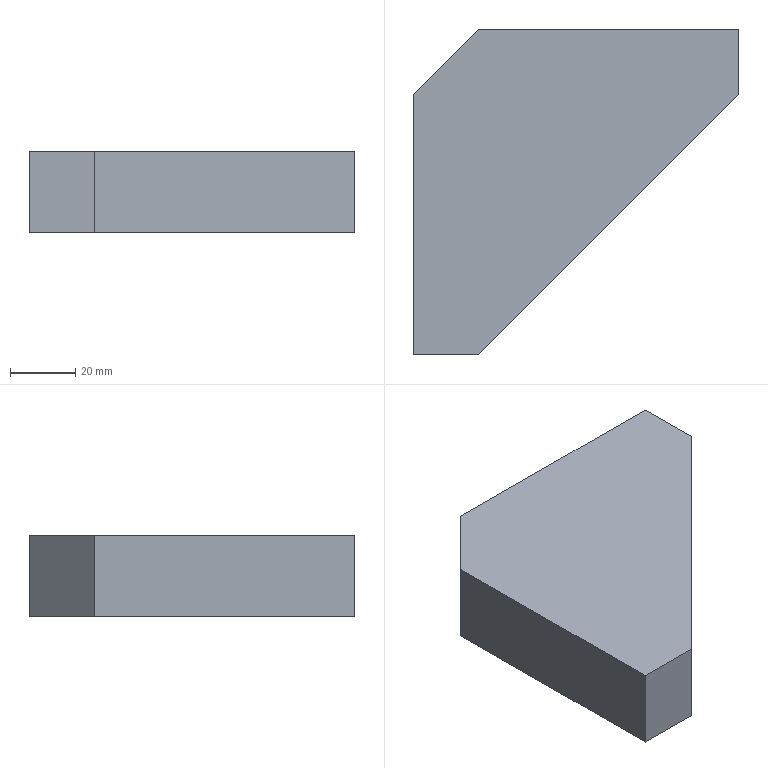Part | SolidWorks | features Extrusion 1 | 1 solid | 8 faces | box 100 x 100 x 25 mm | volume 165000 mm3 | plane 8
STEP:
#1=CARTESIAN_POINT('',(0.,80.,0.));
#2=VERTEX_POINT('',#1);
#3=CARTESIAN_POINT('',(0.,0.,0.));
#4=VERTEX_POINT('',#3);
#5=CARTESIAN_POINT('',(0.,80.,0.));
#6=DIRECTION('',(0.,-1.,0.));
#7=VECTOR('',#6,1000.);
#8=LINE('',#5,#7);
#9=EDGE_CURVE('',#2,#4,#8,.T.);
#10=ORIENTED_EDGE('',*,*,#9,.T.);
#11=CARTESIAN_POINT('',(0.,0.,25.));
#12=VERTEX_POINT('',#11);
#13=CARTESIAN_POINT('',(0.,0.,25.));
#14=DIRECTION('',(0.,0.,-1.));
#15=VECTOR('',#14,1000.);
#16=LINE('',#13,#15);
#17=EDGE_CURVE('',#12,#4,#16,.T.);
#18=ORIENTED_EDGE('',*,*,#17,.F.);
#19=CARTESIAN_POINT('',(0.,80.,25.));
#20=VERTEX_POINT('',#19);
#21=CARTESIAN_POINT('',(0.,80.,25.));
#22=DIRECTION('',(0.,-1.,0.));
#23=VECTOR('',#22,1000.);
#24=LINE('',#21,#23);
#25=EDGE_CURVE('',#20,#12,#24,.T.);
#26=ORIENTED_EDGE('',*,*,#25,.F.);
#27=CARTESIAN_POINT('',(0.,80.,25.));
#28=DIRECTION('',(0.,0.,-1.));
#29=VECTOR('',#28,1000.);
#30=LINE('',#27,#29);
#31=EDGE_CURVE('',#20,#2,#30,.T.);
#32=ORIENTED_EDGE('',*,*,#31,.T.);
#33=EDGE_LOOP('',(#10,#18,#26,#32));
#34=FACE_OUTER_BOUND('',#33,.T.);
#35=CARTESIAN_POINT('',(0.,80.,25.));
#36=DIRECTION('',(1.,0.,0.));
#37=DIRECTION('',(0.,1.,0.));
#38=AXIS2_PLACEMENT_3D('',#35,#36,#37);
#39=PLANE('',#38);
#40=ADVANCED_FACE('',(#34),#39,.F.);
#41=CARTESIAN_POINT('',(20.,0.,0.));
#42=VERTEX_POINT('',#41);
#43=CARTESIAN_POINT('',(0.,0.,0.));
#44=DIRECTION('',(1.,0.,0.));
#45=VECTOR('',#44,1000.);
#46=LINE('',#43,#45);
#47=EDGE_CURVE('',#4,#42,#46,.T.);
#48=ORIENTED_EDGE('',*,*,#47,.T.);
#49=CARTESIAN_POINT('',(20.,0.,25.));
#50=VERTEX_POINT('',#49);
#51=CARTESIAN_POINT('',(20.,0.,25.));
#52=DIRECTION('',(0.,0.,-1.));
#53=VECTOR('',#52,1000.);
#54=LINE('',#51,#53);
#55=EDGE_CURVE('',#50,#42,#54,.T.);
#56=ORIENTED_EDGE('',*,*,#55,.F.);
#57=CARTESIAN_POINT('',(0.,0.,25.));
#58=DIRECTION('',(1.,0.,0.));
#59=VECTOR('',#58,1000.);
#60=LINE('',#57,#59);
#61=EDGE_CURVE('',#12,#50,#60,.T.);
#62=ORIENTED_EDGE('',*,*,#61,.F.);
#63=ORIENTED_EDGE('',*,*,#17,.T.);
#64=EDGE_LOOP('',(#48,#56,#62,#63));
#65=FACE_OUTER_BOUND('',#64,.T.);
#66=CARTESIAN_POINT('',(0.,0.,25.));
#67=DIRECTION('',(0.,1.,0.));
#68=DIRECTION('',(0.,0.,1.));
#69=AXIS2_PLACEMENT_3D('',#66,#67,#68);
#70=PLANE('',#69);
#71=ADVANCED_FACE('',(#65),#70,.F.);
#72=CARTESIAN_POINT('',(100.,80.,0.));
#73=VERTEX_POINT('',#72);
#74=CARTESIAN_POINT('',(20.,0.,0.));
#75=DIRECTION('',(0.7071,0.7071,0.));
#76=VECTOR('',#75,1000.);
#77=LINE('',#74,#76);
#78=EDGE_CURVE('',#42,#73,#77,.T.);
#79=ORIENTED_EDGE('',*,*,#78,.T.);
#80=CARTESIAN_POINT('',(100.,80.,25.));
#81=VERTEX_POINT('',#80);
#82=CARTESIAN_POINT('',(100.,80.,25.));
#83=DIRECTION('',(0.,0.,-1.));
#84=VECTOR('',#83,1000.);
#85=LINE('',#82,#84);
#86=EDGE_CURVE('',#81,#73,#85,.T.);
#87=ORIENTED_EDGE('',*,*,#86,.F.);
#88=CARTESIAN_POINT('',(20.,0.,25.));
#89=DIRECTION('',(0.7071,0.7071,0.));
#90=VECTOR('',#89,1000.);
#91=LINE('',#88,#90);
#92=EDGE_CURVE('',#50,#81,#91,.T.);
#93=ORIENTED_EDGE('',*,*,#92,.F.);
#94=ORIENTED_EDGE('',*,*,#55,.T.);
#95=EDGE_LOOP('',(#79,#87,#93,#94));
#96=FACE_OUTER_BOUND('',#95,.T.);
#97=CARTESIAN_POINT('',(20.,0.,25.));
#98=DIRECTION('',(-0.7071,0.7071,0.));
#99=DIRECTION('',(-0.7071,-0.7071,0.));
#100=AXIS2_PLACEMENT_3D('',#97,#98,#99);
#101=PLANE('',#100);
#102=ADVANCED_FACE('',(#96),#101,.F.);
#103=CARTESIAN_POINT('',(100.,100.,0.));
#104=VERTEX_POINT('',#103);
#105=CARTESIAN_POINT('',(100.,80.,0.));
#106=DIRECTION('',(0.,1.,0.));
#107=VECTOR('',#106,1000.);
#108=LINE('',#105,#107);
#109=EDGE_CURVE('',#73,#104,#108,.T.);
#110=ORIENTED_EDGE('',*,*,#109,.T.);
#111=CARTESIAN_POINT('',(100.,100.,25.));
#112=VERTEX_POINT('',#111);
#113=CARTESIAN_POINT('',(100.,100.,25.));
#114=DIRECTION('',(0.,0.,-1.));
#115=VECTOR('',#114,1000.);
#116=LINE('',#113,#115);
#117=EDGE_CURVE('',#112,#104,#116,.T.);
#118=ORIENTED_EDGE('',*,*,#117,.F.);
#119=CARTESIAN_POINT('',(100.,80.,25.));
#120=DIRECTION('',(0.,1.,0.));
#121=VECTOR('',#120,1000.);
#122=LINE('',#119,#121);
#123=EDGE_CURVE('',#81,#112,#122,.T.);
#124=ORIENTED_EDGE('',*,*,#123,.F.);
#125=ORIENTED_EDGE('',*,*,#86,.T.);
#126=EDGE_LOOP('',(#110,#118,#124,#125));
#127=FACE_OUTER_BOUND('',#126,.T.);
#128=CARTESIAN_POINT('',(100.,80.,25.));
#129=DIRECTION('',(-1.,0.,0.));
#130=DIRECTION('',(0.,0.,1.));
#131=AXIS2_PLACEMENT_3D('',#128,#129,#130);
#132=PLANE('',#131);
#133=ADVANCED_FACE('',(#127),#132,.F.);
#134=CARTESIAN_POINT('',(20.,100.,0.));
#135=VERTEX_POINT('',#134);
#136=CARTESIAN_POINT('',(100.,100.,0.));
#137=DIRECTION('',(-1.,0.,0.));
#138=VECTOR('',#137,1000.);
#139=LINE('',#136,#138);
#140=EDGE_CURVE('',#104,#135,#139,.T.);
#141=ORIENTED_EDGE('',*,*,#140,.T.);
#142=CARTESIAN_POINT('',(20.,100.,25.));
#143=VERTEX_POINT('',#142);
#144=CARTESIAN_POINT('',(20.,100.,25.));
#145=DIRECTION('',(0.,0.,-1.));
#146=VECTOR('',#145,1000.);
#147=LINE('',#144,#146);
#148=EDGE_CURVE('',#143,#135,#147,.T.);
#149=ORIENTED_EDGE('',*,*,#148,.F.);
#150=CARTESIAN_POINT('',(100.,100.,25.));
#151=DIRECTION('',(-1.,0.,0.));
#152=VECTOR('',#151,1000.);
#153=LINE('',#150,#152);
#154=EDGE_CURVE('',#112,#143,#153,.T.);
#155=ORIENTED_EDGE('',*,*,#154,.F.);
#156=ORIENTED_EDGE('',*,*,#117,.T.);
#157=EDGE_LOOP('',(#141,#149,#155,#156));
#158=FACE_OUTER_BOUND('',#157,.T.);
#159=CARTESIAN_POINT('',(100.,100.,25.));
#160=DIRECTION('',(0.,-1.,0.));
#161=DIRECTION('',(1.,0.,0.));
#162=AXIS2_PLACEMENT_3D('',#159,#160,#161);
#163=PLANE('',#162);
#164=ADVANCED_FACE('',(#158),#163,.F.);
#165=CARTESIAN_POINT('',(20.,100.,0.));
#166=DIRECTION('',(-0.7071,-0.7071,0.));
#167=VECTOR('',#166,1000.);
#168=LINE('',#165,#167);
#169=EDGE_CURVE('',#135,#2,#168,.T.);
#170=ORIENTED_EDGE('',*,*,#169,.T.);
#171=ORIENTED_EDGE('',*,*,#31,.F.);
#172=CARTESIAN_POINT('',(20.,100.,25.));
#173=DIRECTION('',(-0.7071,-0.7071,0.));
#174=VECTOR('',#173,1000.);
#175=LINE('',#172,#174);
#176=EDGE_CURVE('',#143,#20,#175,.T.);
#177=ORIENTED_EDGE('',*,*,#176,.F.);
#178=ORIENTED_EDGE('',*,*,#148,.T.);
#179=EDGE_LOOP('',(#170,#171,#177,#178));
#180=FACE_OUTER_BOUND('',#179,.T.);
#181=CARTESIAN_POINT('',(20.,100.,25.));
#182=DIRECTION('',(0.7071,-0.7071,0.));
#183=DIRECTION('',(0.7071,0.7071,0.));
#184=AXIS2_PLACEMENT_3D('',#181,#182,#183);
#185=PLANE('',#184);
#186=ADVANCED_FACE('',(#180),#185,.F.);
#187=ORIENTED_EDGE('',*,*,#25,.T.);
#188=ORIENTED_EDGE('',*,*,#61,.T.);
#189=ORIENTED_EDGE('',*,*,#92,.T.);
#190=ORIENTED_EDGE('',*,*,#123,.T.);
#191=ORIENTED_EDGE('',*,*,#154,.T.);
#192=ORIENTED_EDGE('',*,*,#176,.T.);
#193=EDGE_LOOP('',(#187,#188,#189,#190,#191,#192));
#194=FACE_OUTER_BOUND('',#193,.T.);
#195=CARTESIAN_POINT('',(0.,0.,25.));
#196=DIRECTION('',(0.,0.,1.));
#197=DIRECTION('',(1.,0.,0.));
#198=AXIS2_PLACEMENT_3D('',#195,#196,#197);
#199=PLANE('',#198);
#200=ADVANCED_FACE('',(#194),#199,.T.);
#201=ORIENTED_EDGE('',*,*,#9,.F.);
#202=ORIENTED_EDGE('',*,*,#169,.F.);
#203=ORIENTED_EDGE('',*,*,#140,.F.);
#204=ORIENTED_EDGE('',*,*,#109,.F.);
#205=ORIENTED_EDGE('',*,*,#78,.F.);
#206=ORIENTED_EDGE('',*,*,#47,.F.);
#207=EDGE_LOOP('',(#201,#202,#203,#204,#205,#206));
#208=FACE_OUTER_BOUND('',#207,.T.);
#209=CARTESIAN_POINT('',(0.,0.,0.));
#210=DIRECTION('',(0.,0.,1.));
#211=DIRECTION('',(1.,0.,0.));
#212=AXIS2_PLACEMENT_3D('',#209,#210,#211);
#213=PLANE('',#212);
#214=ADVANCED_FACE('',(#208),#213,.F.);
#215=CLOSED_SHELL('',(#40,#71,#102,#133,#164,#186,#200,#214));
#216=MANIFOLD_SOLID_BREP('',#215);
#217=CARTESIAN_POINT('',(0.,0.,0.));
#218=DIRECTION('',(0.,0.,1.));
#219=DIRECTION('',(1.,0.,0.));
#220=AXIS2_PLACEMENT_3D('',#217,#218,#219);
#221=(LENGTH_UNIT()NAMED_UNIT(*)SI_UNIT(.MILLI.,.METRE.));
#222=UNCERTAINTY_MEASURE_WITH_UNIT(LENGTH_MEASURE(0.00001),#221,'','');
#223=(NAMED_UNIT(*)PLANE_ANGLE_UNIT()SI_UNIT($,.RADIAN.));
#224=(NAMED_UNIT(*)SI_UNIT($,.STERADIAN.)SOLID_ANGLE_UNIT());
#225=(GEOMETRIC_REPRESENTATION_CONTEXT(3)GLOBAL_UNCERTAINTY_ASSIGNED_CONTEXT((#222))GLOBAL_UNIT_ASSIGNED_CONTEXT((#221,#223,#224))REPRESENTATION_CONTEXT('',''));
#226=ADVANCED_BREP_SHAPE_REPRESENTATION('',(#216,#220),#225);